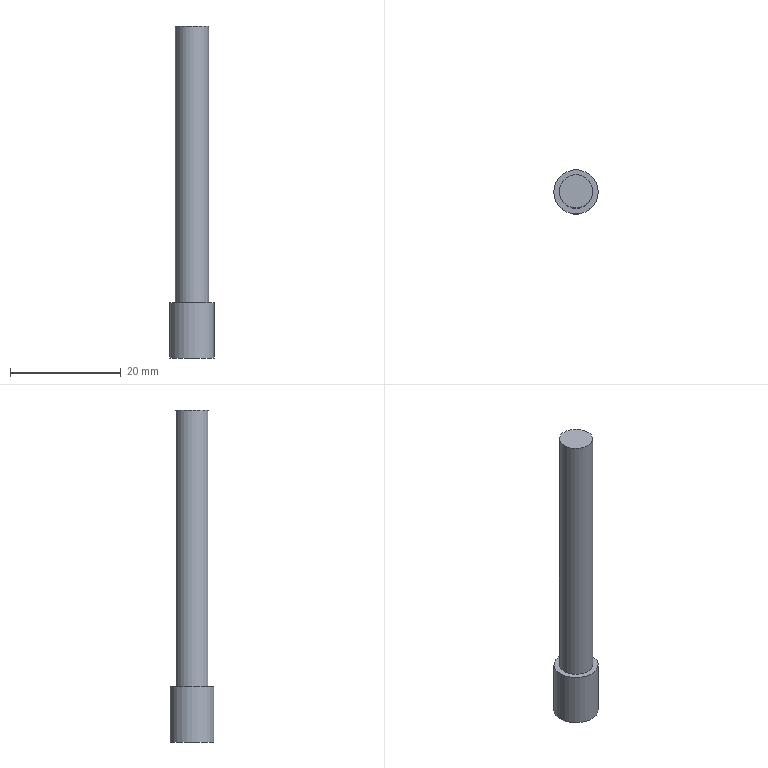Part | NX | features solid 2 | 1 solid | 5 faces | box 8 x 8 x 60 mm | volume 1916 mm3 | plane 3 | cylinder 2 | commonest cylinder face diameters 6 x1 8 x1
STEP:
#1=CARTESIAN_POINT('',(-64.,-32.,10.));
#2=VERTEX_POINT('',#1);
#3=CARTESIAN_POINT('',(-67.,-32.,10.));
#4=DIRECTION('',(0.,0.,1.));
#5=DIRECTION('',(1.,0.,0.));
#6=AXIS2_PLACEMENT_3D('',#3,#4,#5);
#7=CIRCLE('',#6,3.);
#8=EDGE_CURVE('',#2,#2,#7,.T.);
#9=ORIENTED_EDGE('',*,*,#8,.F.);
#10=EDGE_LOOP('',(#9));
#11=FACE_BOUND('',#10,.T.);
#12=CARTESIAN_POINT('',(-64.,-32.,-40.));
#13=VERTEX_POINT('',#12);
#14=CARTESIAN_POINT('',(-67.,-32.,-40.));
#15=DIRECTION('',(0.,0.,1.));
#16=DIRECTION('',(1.,0.,0.));
#17=AXIS2_PLACEMENT_3D('',#14,#15,#16);
#18=CIRCLE('',#17,3.);
#19=EDGE_CURVE('',#13,#13,#18,.F.);
#20=ORIENTED_EDGE('',*,*,#19,.F.);
#21=EDGE_LOOP('',(#20));
#22=FACE_BOUND('',#21,.T.);
#23=CARTESIAN_POINT('',(-67.,-32.,-35.));
#24=DIRECTION('',(0.,0.,1.));
#25=DIRECTION('',(-1.,0.,0.));
#26=AXIS2_PLACEMENT_3D('',#23,#24,#25);
#27=CYLINDRICAL_SURFACE('',#26,3.);
#28=ADVANCED_FACE('',(#11,#22),#27,.T.);
#29=ORIENTED_EDGE('',*,*,#8,.T.);
#30=EDGE_LOOP('',(#29));
#31=FACE_BOUND('',#30,.T.);
#32=CARTESIAN_POINT('',(-67.,-32.,10.));
#33=DIRECTION('',(0.,0.,1.));
#34=DIRECTION('',(-1.,0.,0.));
#35=AXIS2_PLACEMENT_3D('',#32,#33,#34);
#36=PLANE('',#35);
#37=ADVANCED_FACE('',(#31),#36,.T.);
#38=CARTESIAN_POINT('',(-63.,-32.,-40.));
#39=VERTEX_POINT('',#38);
#40=CARTESIAN_POINT('',(-67.,-32.,-40.));
#41=DIRECTION('',(0.,0.,1.));
#42=DIRECTION('',(1.,0.,0.));
#43=AXIS2_PLACEMENT_3D('',#40,#41,#42);
#44=CIRCLE('',#43,4.);
#45=EDGE_CURVE('',#39,#39,#44,.T.);
#46=ORIENTED_EDGE('',*,*,#45,.F.);
#47=EDGE_LOOP('',(#46));
#48=FACE_BOUND('',#47,.T.);
#49=CARTESIAN_POINT('',(-63.,-32.,-50.));
#50=VERTEX_POINT('',#49);
#51=CARTESIAN_POINT('',(-67.,-32.,-50.));
#52=DIRECTION('',(0.,0.,1.));
#53=DIRECTION('',(1.,0.,0.));
#54=AXIS2_PLACEMENT_3D('',#51,#52,#53);
#55=CIRCLE('',#54,4.);
#56=EDGE_CURVE('',#50,#50,#55,.T.);
#57=ORIENTED_EDGE('',*,*,#56,.T.);
#58=EDGE_LOOP('',(#57));
#59=FACE_BOUND('',#58,.T.);
#60=CARTESIAN_POINT('',(-67.,-32.,-38.));
#61=DIRECTION('',(0.,0.,-1.));
#62=DIRECTION('',(1.,0.,0.));
#63=AXIS2_PLACEMENT_3D('',#60,#61,#62);
#64=CYLINDRICAL_SURFACE('',#63,4.);
#65=ADVANCED_FACE('',(#48,#59),#64,.T.);
#66=ORIENTED_EDGE('',*,*,#19,.T.);
#67=EDGE_LOOP('',(#66));
#68=FACE_BOUND('',#67,.T.);
#69=ORIENTED_EDGE('',*,*,#45,.T.);
#70=EDGE_LOOP('',(#69));
#71=FACE_BOUND('',#70,.T.);
#72=CARTESIAN_POINT('',(-67.,-32.,-40.));
#73=DIRECTION('',(0.,0.,-1.));
#74=DIRECTION('',(1.,0.,0.));
#75=AXIS2_PLACEMENT_3D('',#72,#73,#74);
#76=PLANE('',#75);
#77=ADVANCED_FACE('',(#68,#71),#76,.F.);
#78=ORIENTED_EDGE('',*,*,#56,.F.);
#79=EDGE_LOOP('',(#78));
#80=FACE_BOUND('',#79,.T.);
#81=CARTESIAN_POINT('',(-8.802,-9.836,-50.));
#82=DIRECTION('',(0.,0.,1.));
#83=DIRECTION('',(1.,0.,0.));
#84=AXIS2_PLACEMENT_3D('',#81,#82,#83);
#85=PLANE('',#84);
#86=ADVANCED_FACE('',(#80),#85,.F.);
#87=CLOSED_SHELL('',(#28,#37,#65,#77,#86));
#88=MANIFOLD_SOLID_BREP('',#87);
#89=(LENGTH_UNIT()NAMED_UNIT(*)SI_UNIT(.MILLI.,.METRE.));
#90=UNCERTAINTY_MEASURE_WITH_UNIT(LENGTH_MEASURE(0.00001),#89,'','');
#91=(NAMED_UNIT(*)PLANE_ANGLE_UNIT()SI_UNIT($,.RADIAN.));
#92=(NAMED_UNIT(*)SI_UNIT($,.STERADIAN.)SOLID_ANGLE_UNIT());
#93=(GEOMETRIC_REPRESENTATION_CONTEXT(3)GLOBAL_UNCERTAINTY_ASSIGNED_CONTEXT((#90))GLOBAL_UNIT_ASSIGNED_CONTEXT((#89,#91,#92))REPRESENTATION_CONTEXT('',''));
#94=ADVANCED_BREP_SHAPE_REPRESENTATION('',(#88),#93);